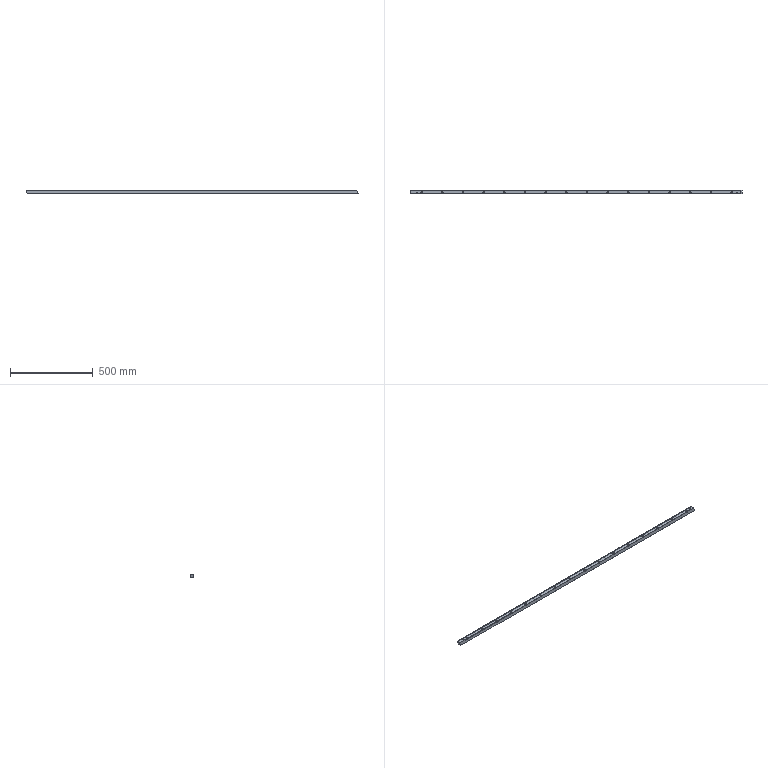Part | SolidWorks | features ICE 10, BaseBody 1, LPattern 1, MoveFace 1 | 1 solid | 1891 faces | box 2009 x 24 x 24 mm | volume 1024177 mm3 | plane 1823 | cylinder 68 | commonest cylinder face diameters 7 x32 11 x32 5.7 x4